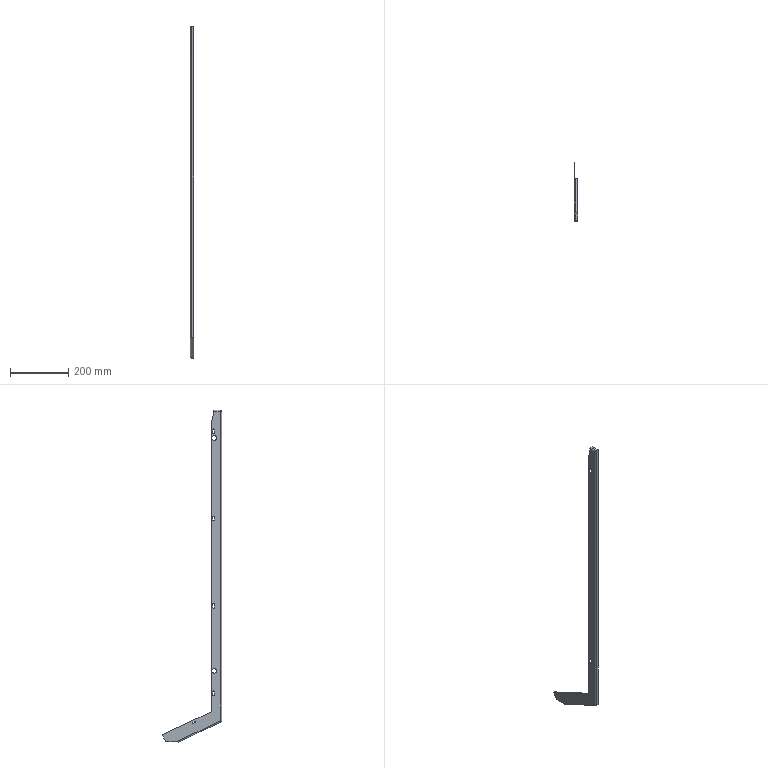Part | NX | features solid 2 | 1 solid | 64 faces | box 12 x 203.72 x 1140 mm | volume 112703 mm3 | plane 38 | cylinder 25 | spline 1 | commonest cylinder face diameters 6 x12 16 x4 4 x3 5 x3 8 x3